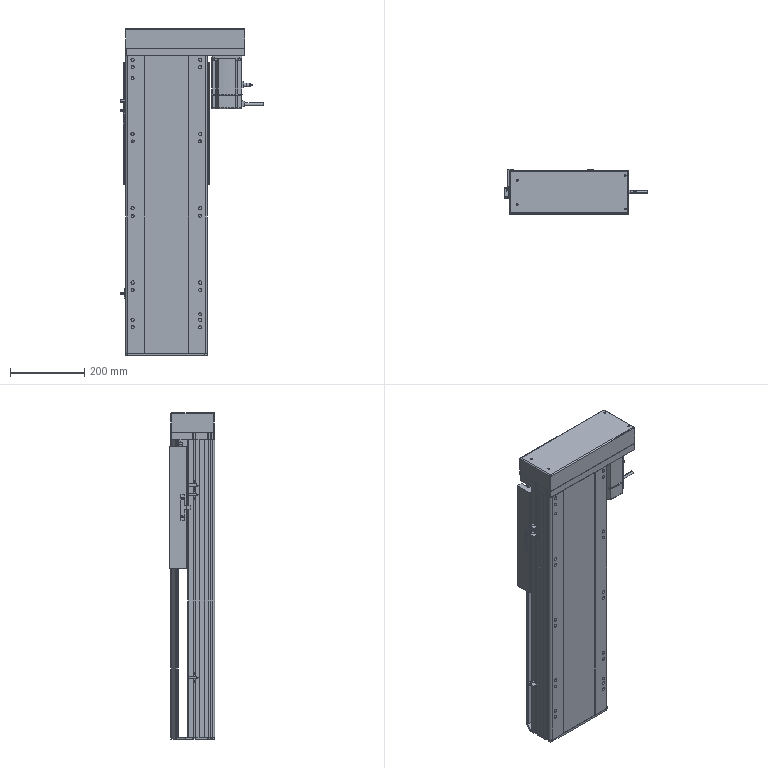Part | SolidWorks | features BaseBody 11 | 11 solids | 1541 faces | box 384.7 x 122 x 879.7 mm | volume 13861724 mm3 | plane 777 | cylinder 429 | spline 228 | cone 56 | torus 35 | sphere 16 | commonest cylinder face diameters 2 x60 0.6 x48 1 x48 14 x24 3.3 x20 8.5 x20